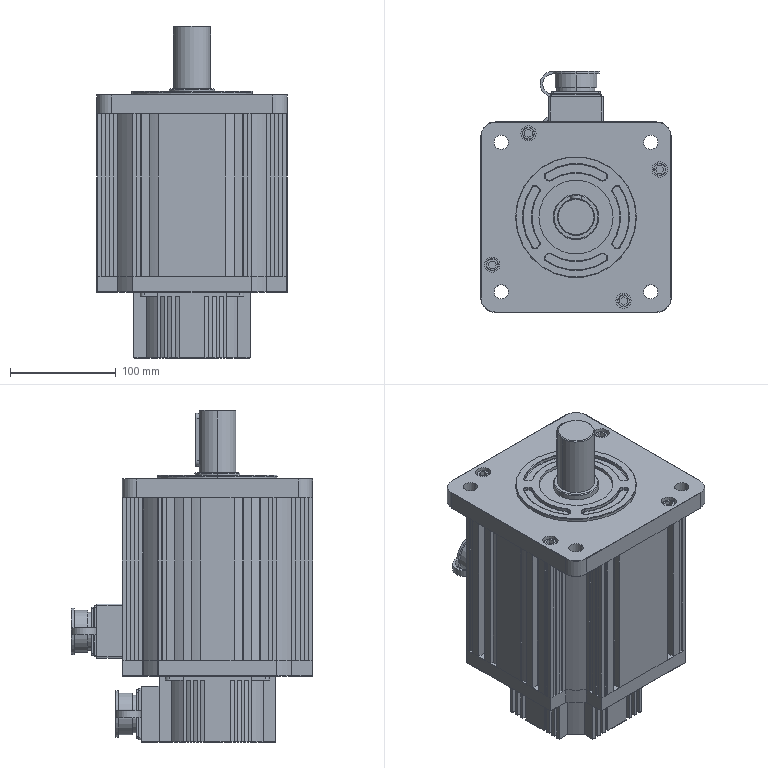Part | SolidWorks | features ICE 33, Fillet 11, MirrorPattern 7, CirPattern 5, Extrusion 3, Revolution 3, Chamfer 2, Sweep 2, PLine 1 | 1 solid | 1306 faces | box 180 x 228 x 314 mm | volume 6100374 mm3 | plane 565 | cylinder 527 | torus 192 | sphere 16 | cone 6 | commonest cylinder face diameters 0.4 x289 108 x28 6.858 x20 180 x20 0.64 x16 3.6 x16